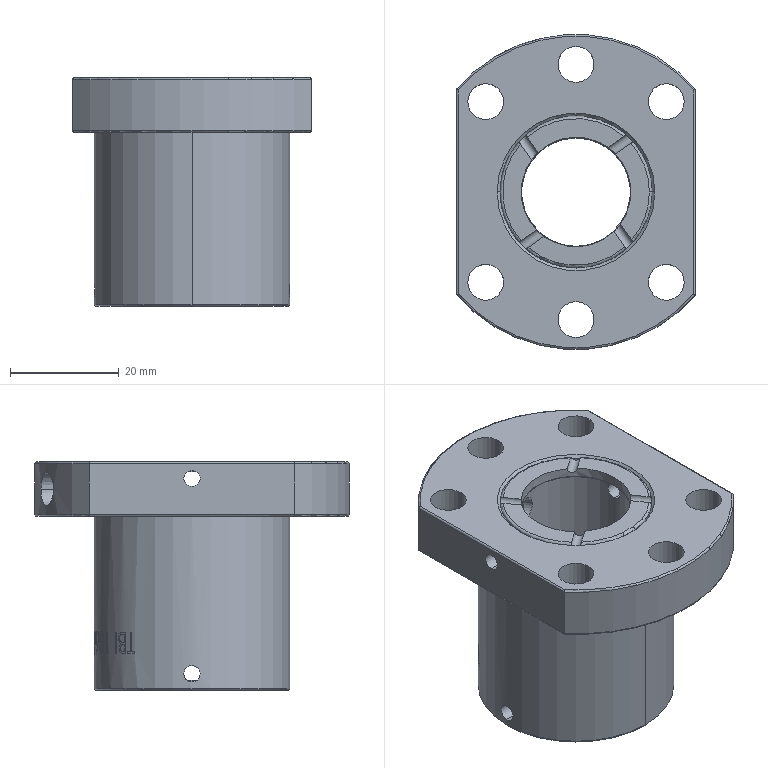Part | STEP file | 3 solids | 281 faces | box 44 x 58 x 42 mm | volume 39340 mm3 | spline 120 | cylinder 82 | plane 59 | torus 16 | cone 4 | commonest cylinder face diameters 36 x15 36.02 x15 6.6 x12 1.8 x8 3 x8 28 x8